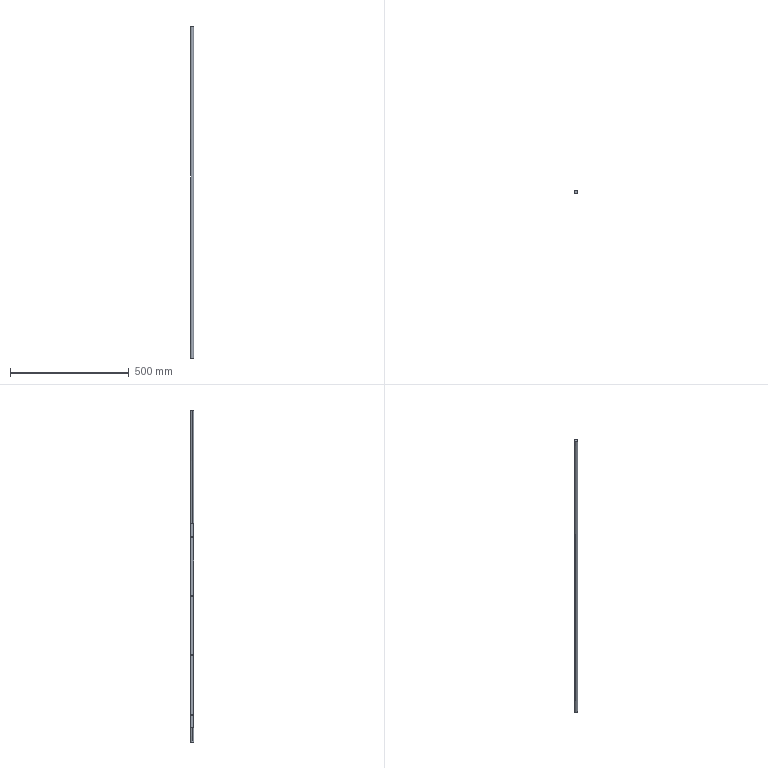Part | STEP file | 1 solid | 15 faces | box 14 x 14 x 1400 mm | volume 203252 mm3 | cylinder 10 | plane 5 | commonest cylinder face diameters 4.2 x8 14 x2